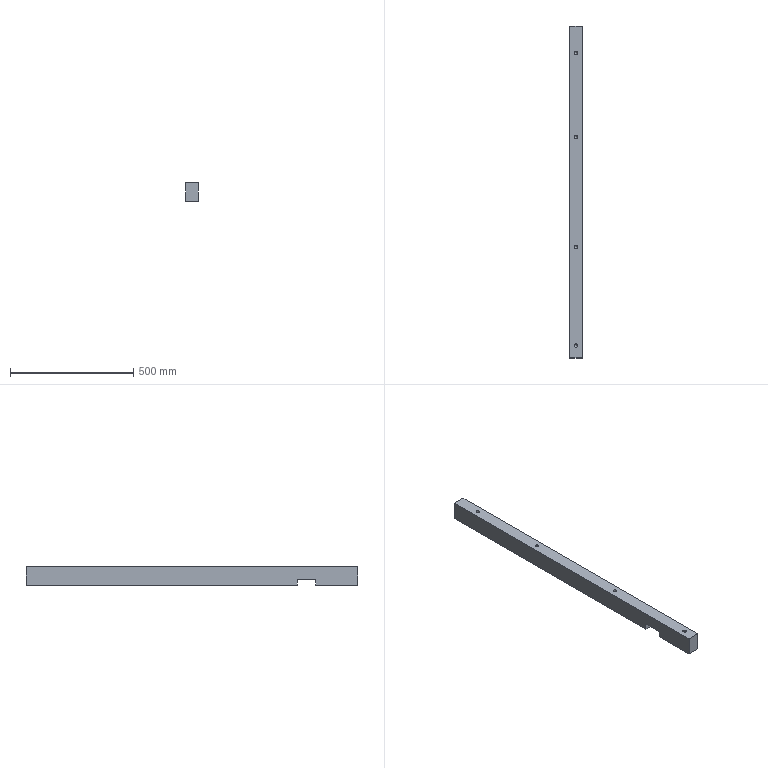Part | NX | features 3 2 | 1 solid | 26 faces | box 50 x 1345 x 75.5 mm | volume 4973309 mm3 | plane 10 | cylinder 8 | cone 8 | commonest cylinder face diameters 14.1 x8
STEP:
#1=CARTESIAN_POINT('',(3150.05,222.5,256.5));
#2=VERTEX_POINT('',#1);
#3=CARTESIAN_POINT('',(3143.,222.5,256.5));
#4=DIRECTION('',(0.,0.,-1.));
#5=DIRECTION('',(1.,0.,0.));
#6=AXIS2_PLACEMENT_3D('',#3,#4,#5);
#7=CIRCLE('',#6,7.05);
#8=EDGE_CURVE('',#2,#2,#7,.T.);
#9=ORIENTED_EDGE('',*,*,#8,.T.);
#10=EDGE_LOOP('',(#9));
#11=FACE_BOUND('',#10,.T.);
#12=CARTESIAN_POINT('',(3150.05,-222.5,256.5));
#13=VERTEX_POINT('',#12);
#14=CARTESIAN_POINT('',(3143.,-222.5,256.5));
#15=DIRECTION('',(0.,0.,-1.));
#16=DIRECTION('',(1.,0.,0.));
#17=AXIS2_PLACEMENT_3D('',#14,#15,#16);
#18=CIRCLE('',#17,7.05);
#19=EDGE_CURVE('',#13,#13,#18,.T.);
#20=ORIENTED_EDGE('',*,*,#19,.T.);
#21=EDGE_LOOP('',(#20));
#22=FACE_BOUND('',#21,.T.);
#23=CARTESIAN_POINT('',(3168.,-672.5,256.5));
#24=VERTEX_POINT('',#23);
#25=CARTESIAN_POINT('',(3168.,672.5,256.5));
#26=VERTEX_POINT('',#25);
#27=CARTESIAN_POINT('',(3168.,193.,256.5));
#28=DIRECTION('',(0.,1.,0.));
#29=VECTOR('',#28,1000.);
#30=LINE('',#27,#29);
#31=EDGE_CURVE('',#24,#26,#30,.T.);
#32=ORIENTED_EDGE('',*,*,#31,.T.);
#33=CARTESIAN_POINT('',(3118.,672.5,256.5));
#34=VERTEX_POINT('',#33);
#35=CARTESIAN_POINT('',(1128.,672.5,256.5));
#36=DIRECTION('',(-1.,0.,0.));
#37=VECTOR('',#36,1000.);
#38=LINE('',#35,#37);
#39=EDGE_CURVE('',#26,#34,#38,.T.);
#40=ORIENTED_EDGE('',*,*,#39,.T.);
#41=CARTESIAN_POINT('',(3118.,-672.5,256.5));
#42=VERTEX_POINT('',#41);
#43=CARTESIAN_POINT('',(3118.,193.,256.5));
#44=DIRECTION('',(0.,-1.,0.));
#45=VECTOR('',#44,1000.);
#46=LINE('',#43,#45);
#47=EDGE_CURVE('',#34,#42,#46,.T.);
#48=ORIENTED_EDGE('',*,*,#47,.T.);
#49=CARTESIAN_POINT('',(1128.,-672.5,256.5));
#50=DIRECTION('',(1.,0.,0.));
#51=VECTOR('',#50,1000.);
#52=LINE('',#49,#51);
#53=EDGE_CURVE('',#42,#24,#52,.T.);
#54=ORIENTED_EDGE('',*,*,#53,.T.);
#55=EDGE_LOOP('',(#32,#40,#48,#54));
#56=FACE_BOUND('',#55,.T.);
#57=CARTESIAN_POINT('',(3150.05,-622.5,256.5));
#58=VERTEX_POINT('',#57);
#59=CARTESIAN_POINT('',(3143.,-622.5,256.5));
#60=DIRECTION('',(0.,0.,-1.));
#61=DIRECTION('',(1.,0.,0.));
#62=AXIS2_PLACEMENT_3D('',#59,#60,#61);
#63=CIRCLE('',#62,7.05);
#64=EDGE_CURVE('',#58,#58,#63,.T.);
#65=ORIENTED_EDGE('',*,*,#64,.T.);
#66=EDGE_LOOP('',(#65));
#67=FACE_BOUND('',#66,.T.);
#68=CARTESIAN_POINT('',(3150.05,562.5,256.5));
#69=VERTEX_POINT('',#68);
#70=CARTESIAN_POINT('',(3143.,562.5,256.5));
#71=DIRECTION('',(0.,0.,-1.));
#72=DIRECTION('',(1.,0.,0.));
#73=AXIS2_PLACEMENT_3D('',#70,#71,#72);
#74=CIRCLE('',#73,7.05);
#75=EDGE_CURVE('',#69,#69,#74,.T.);
#76=ORIENTED_EDGE('',*,*,#75,.T.);
#77=EDGE_LOOP('',(#76));
#78=FACE_BOUND('',#77,.T.);
#79=CARTESIAN_POINT('',(1128.,0.,256.5));
#80=DIRECTION('',(0.,0.,1.));
#81=DIRECTION('',(1.,0.,0.));
#82=AXIS2_PLACEMENT_3D('',#79,#80,#81);
#83=PLANE('',#82);
#84=ADVANCED_FACE('',(#11,#22,#56,#67,#78),#83,.T.);
#85=CARTESIAN_POINT('',(3150.05,-222.5,181.));
#86=VERTEX_POINT('',#85);
#87=CARTESIAN_POINT('',(3143.,-222.5,181.));
#88=DIRECTION('',(0.,0.,1.));
#89=DIRECTION('',(1.,0.,0.));
#90=AXIS2_PLACEMENT_3D('',#87,#88,#89);
#91=CIRCLE('',#90,7.05);
#92=EDGE_CURVE('',#86,#86,#91,.T.);
#93=ORIENTED_EDGE('',*,*,#92,.T.);
#94=EDGE_LOOP('',(#93));
#95=FACE_BOUND('',#94,.T.);
#96=CARTESIAN_POINT('',(3118.,-426.,181.));
#97=VERTEX_POINT('',#96);
#98=CARTESIAN_POINT('',(3168.,-426.,181.));
#99=VERTEX_POINT('',#98);
#100=CARTESIAN_POINT('',(1898.,-426.,181.));
#101=DIRECTION('',(1.,0.,0.));
#102=VECTOR('',#101,1000.);
#103=LINE('',#100,#102);
#104=EDGE_CURVE('',#97,#99,#103,.T.);
#105=ORIENTED_EDGE('',*,*,#104,.F.);
#106=CARTESIAN_POINT('',(3118.,672.5,181.));
#107=VERTEX_POINT('',#106);
#108=CARTESIAN_POINT('',(3118.,193.,181.));
#109=DIRECTION('',(0.,1.,0.));
#110=VECTOR('',#109,1000.);
#111=LINE('',#108,#110);
#112=EDGE_CURVE('',#97,#107,#111,.T.);
#113=ORIENTED_EDGE('',*,*,#112,.T.);
#114=CARTESIAN_POINT('',(3168.,672.5,181.));
#115=VERTEX_POINT('',#114);
#116=CARTESIAN_POINT('',(3168.,672.5,181.));
#117=DIRECTION('',(-1.,0.,0.));
#118=VECTOR('',#117,1000.);
#119=LINE('',#116,#118);
#120=EDGE_CURVE('',#115,#107,#119,.T.);
#121=ORIENTED_EDGE('',*,*,#120,.F.);
#122=CARTESIAN_POINT('',(3168.,193.,181.));
#123=DIRECTION('',(0.,-1.,0.));
#124=VECTOR('',#123,1000.);
#125=LINE('',#122,#124);
#126=EDGE_CURVE('',#115,#99,#125,.T.);
#127=ORIENTED_EDGE('',*,*,#126,.T.);
#128=EDGE_LOOP('',(#105,#113,#121,#127));
#129=FACE_BOUND('',#128,.T.);
#130=CARTESIAN_POINT('',(3150.05,222.5,181.));
#131=VERTEX_POINT('',#130);
#132=CARTESIAN_POINT('',(3143.,222.5,181.));
#133=DIRECTION('',(0.,0.,1.));
#134=DIRECTION('',(1.,0.,0.));
#135=AXIS2_PLACEMENT_3D('',#132,#133,#134);
#136=CIRCLE('',#135,7.05);
#137=EDGE_CURVE('',#131,#131,#136,.T.);
#138=ORIENTED_EDGE('',*,*,#137,.T.);
#139=EDGE_LOOP('',(#138));
#140=FACE_BOUND('',#139,.T.);
#141=CARTESIAN_POINT('',(3150.05,562.5,181.));
#142=VERTEX_POINT('',#141);
#143=CARTESIAN_POINT('',(3143.,562.5,181.));
#144=DIRECTION('',(0.,0.,1.));
#145=DIRECTION('',(1.,0.,0.));
#146=AXIS2_PLACEMENT_3D('',#143,#144,#145);
#147=CIRCLE('',#146,7.05);
#148=EDGE_CURVE('',#142,#142,#147,.T.);
#149=ORIENTED_EDGE('',*,*,#148,.T.);
#150=EDGE_LOOP('',(#149));
#151=FACE_BOUND('',#150,.T.);
#152=CARTESIAN_POINT('',(1898.,193.,181.));
#153=DIRECTION('',(0.,0.,-1.));
#154=DIRECTION('',(1.,0.,0.));
#155=AXIS2_PLACEMENT_3D('',#152,#153,#154);
#156=PLANE('',#155);
#157=ADVANCED_FACE('',(#95,#129,#140,#151),#156,.T.);
#158=CARTESIAN_POINT('',(3168.,-502.,181.));
#159=VERTEX_POINT('',#158);
#160=CARTESIAN_POINT('',(3118.,-502.,181.));
#161=VERTEX_POINT('',#160);
#162=CARTESIAN_POINT('',(1898.,-502.,181.));
#163=DIRECTION('',(-1.,0.,0.));
#164=VECTOR('',#163,1000.);
#165=LINE('',#162,#164);
#166=EDGE_CURVE('',#159,#161,#165,.T.);
#167=ORIENTED_EDGE('',*,*,#166,.F.);
#168=CARTESIAN_POINT('',(3168.,-672.5,181.));
#169=VERTEX_POINT('',#168);
#170=CARTESIAN_POINT('',(3168.,193.,181.));
#171=DIRECTION('',(0.,-1.,0.));
#172=VECTOR('',#171,1000.);
#173=LINE('',#170,#172);
#174=EDGE_CURVE('',#159,#169,#173,.T.);
#175=ORIENTED_EDGE('',*,*,#174,.T.);
#176=CARTESIAN_POINT('',(3118.,-672.5,181.));
#177=VERTEX_POINT('',#176);
#178=CARTESIAN_POINT('',(265.5,-672.5,181.));
#179=DIRECTION('',(1.,0.,0.));
#180=VECTOR('',#179,1000.);
#181=LINE('',#178,#180);
#182=EDGE_CURVE('',#177,#169,#181,.T.);
#183=ORIENTED_EDGE('',*,*,#182,.F.);
#184=CARTESIAN_POINT('',(3118.,193.,181.));
#185=DIRECTION('',(0.,1.,0.));
#186=VECTOR('',#185,1000.);
#187=LINE('',#184,#186);
#188=EDGE_CURVE('',#177,#161,#187,.T.);
#189=ORIENTED_EDGE('',*,*,#188,.T.);
#190=EDGE_LOOP('',(#167,#175,#183,#189));
#191=FACE_BOUND('',#190,.T.);
#192=CARTESIAN_POINT('',(3150.05,-622.5,181.));
#193=VERTEX_POINT('',#192);
#194=CARTESIAN_POINT('',(3143.,-622.5,181.));
#195=DIRECTION('',(0.,0.,1.));
#196=DIRECTION('',(1.,0.,0.));
#197=AXIS2_PLACEMENT_3D('',#194,#195,#196);
#198=CIRCLE('',#197,7.05);
#199=EDGE_CURVE('',#193,#193,#198,.T.);
#200=ORIENTED_EDGE('',*,*,#199,.T.);
#201=EDGE_LOOP('',(#200));
#202=FACE_BOUND('',#201,.T.);
#203=CARTESIAN_POINT('',(1898.,193.,181.));
#204=DIRECTION('',(0.,0.,-1.));
#205=DIRECTION('',(1.,0.,0.));
#206=AXIS2_PLACEMENT_3D('',#203,#204,#205);
#207=PLANE('',#206);
#208=ADVANCED_FACE('',(#191,#202),#207,.T.);
#209=CARTESIAN_POINT('',(3168.,-502.,205.));
#210=VERTEX_POINT('',#209);
#211=CARTESIAN_POINT('',(3168.,-502.,-1.5));
#212=DIRECTION('',(0.,0.,-1.));
#213=VECTOR('',#212,1000.);
#214=LINE('',#211,#213);
#215=EDGE_CURVE('',#210,#159,#214,.T.);
#216=ORIENTED_EDGE('',*,*,#215,.F.);
#217=CARTESIAN_POINT('',(3168.,-426.,205.));
#218=VERTEX_POINT('',#217);
#219=CARTESIAN_POINT('',(3168.,193.,205.));
#220=DIRECTION('',(0.,-1.,0.));
#221=VECTOR('',#220,1000.);
#222=LINE('',#219,#221);
#223=EDGE_CURVE('',#218,#210,#222,.T.);
#224=ORIENTED_EDGE('',*,*,#223,.F.);
#225=CARTESIAN_POINT('',(3168.,-426.,-1.5));
#226=DIRECTION('',(0.,0.,1.));
#227=VECTOR('',#226,1000.);
#228=LINE('',#225,#227);
#229=EDGE_CURVE('',#99,#218,#228,.T.);
#230=ORIENTED_EDGE('',*,*,#229,.F.);
#231=ORIENTED_EDGE('',*,*,#126,.F.);
#232=CARTESIAN_POINT('',(3168.,672.5,231.5));
#233=DIRECTION('',(0.,0.,-1.));
#234=VECTOR('',#233,1000.);
#235=LINE('',#232,#234);
#236=EDGE_CURVE('',#26,#115,#235,.T.);
#237=ORIENTED_EDGE('',*,*,#236,.F.);
#238=ORIENTED_EDGE('',*,*,#31,.F.);
#239=CARTESIAN_POINT('',(3168.,-672.5,-103.));
#240=DIRECTION('',(0.,0.,1.));
#241=VECTOR('',#240,1000.);
#242=LINE('',#239,#241);
#243=EDGE_CURVE('',#169,#24,#242,.T.);
#244=ORIENTED_EDGE('',*,*,#243,.F.);
#245=ORIENTED_EDGE('',*,*,#174,.F.);
#246=EDGE_LOOP('',(#216,#224,#230,#231,#237,#238,#244,#245));
#247=FACE_BOUND('',#246,.T.);
#248=CARTESIAN_POINT('',(3168.,193.,-1.5));
#249=DIRECTION('',(1.,0.,0.));
#250=DIRECTION('',(0.,0.,-1.));
#251=AXIS2_PLACEMENT_3D('',#248,#249,#250);
#252=PLANE('',#251);
#253=ADVANCED_FACE('',(#247),#252,.T.);
#254=CARTESIAN_POINT('',(3118.,-502.,205.));
#255=VERTEX_POINT('',#254);
#256=CARTESIAN_POINT('',(3118.,-502.,-1.5));
#257=DIRECTION('',(0.,0.,1.));
#258=VECTOR('',#257,1000.);
#259=LINE('',#256,#258);
#260=EDGE_CURVE('',#161,#255,#259,.T.);
#261=ORIENTED_EDGE('',*,*,#260,.F.);
#262=ORIENTED_EDGE('',*,*,#188,.F.);
#263=CARTESIAN_POINT('',(3118.,-672.5,-103.));
#264=DIRECTION('',(0.,0.,-1.));
#265=VECTOR('',#264,1000.);
#266=LINE('',#263,#265);
#267=EDGE_CURVE('',#42,#177,#266,.T.);
#268=ORIENTED_EDGE('',*,*,#267,.F.);
#269=ORIENTED_EDGE('',*,*,#47,.F.);
#270=CARTESIAN_POINT('',(3118.,672.5,231.5));
#271=DIRECTION('',(0.,0.,1.));
#272=VECTOR('',#271,1000.);
#273=LINE('',#270,#272);
#274=EDGE_CURVE('',#107,#34,#273,.T.);
#275=ORIENTED_EDGE('',*,*,#274,.F.);
#276=ORIENTED_EDGE('',*,*,#112,.F.);
#277=CARTESIAN_POINT('',(3118.,-426.,205.));
#278=VERTEX_POINT('',#277);
#279=CARTESIAN_POINT('',(3118.,-426.,-1.5));
#280=DIRECTION('',(0.,0.,-1.));
#281=VECTOR('',#280,1000.);
#282=LINE('',#279,#281);
#283=EDGE_CURVE('',#278,#97,#282,.T.);
#284=ORIENTED_EDGE('',*,*,#283,.F.);
#285=CARTESIAN_POINT('',(3118.,193.,205.));
#286=DIRECTION('',(0.,1.,0.));
#287=VECTOR('',#286,1000.);
#288=LINE('',#285,#287);
#289=EDGE_CURVE('',#255,#278,#288,.T.);
#290=ORIENTED_EDGE('',*,*,#289,.F.);
#291=EDGE_LOOP('',(#261,#262,#268,#269,#275,#276,#284,#290));
#292=FACE_BOUND('',#291,.T.);
#293=CARTESIAN_POINT('',(3118.,193.,-1.5));
#294=DIRECTION('',(-1.,0.,0.));
#295=DIRECTION('',(0.,0.,1.));
#296=AXIS2_PLACEMENT_3D('',#293,#294,#295);
#297=PLANE('',#296);
#298=ADVANCED_FACE('',(#292),#297,.T.);
#299=ORIENTED_EDGE('',*,*,#267,.T.);
#300=ORIENTED_EDGE('',*,*,#182,.T.);
#301=ORIENTED_EDGE('',*,*,#243,.T.);
#302=ORIENTED_EDGE('',*,*,#53,.F.);
#303=EDGE_LOOP('',(#299,#300,#301,#302));
#304=FACE_BOUND('',#303,.T.);
#305=CARTESIAN_POINT('',(265.5,-672.5,-103.));
#306=DIRECTION('',(0.,1.,0.));
#307=DIRECTION('',(1.,0.,0.));
#308=AXIS2_PLACEMENT_3D('',#305,#306,#307);
#309=PLANE('',#308);
#310=ADVANCED_FACE('',(#304),#309,.F.);
#311=ORIENTED_EDGE('',*,*,#236,.T.);
#312=ORIENTED_EDGE('',*,*,#120,.T.);
#313=ORIENTED_EDGE('',*,*,#274,.T.);
#314=ORIENTED_EDGE('',*,*,#39,.F.);
#315=EDGE_LOOP('',(#311,#312,#313,#314));
#316=FACE_BOUND('',#315,.T.);
#317=CARTESIAN_POINT('',(3168.,672.5,231.5));
#318=DIRECTION('',(0.,1.,0.));
#319=DIRECTION('',(0.,0.,-1.));
#320=AXIS2_PLACEMENT_3D('',#317,#318,#319);
#321=PLANE('',#320);
#322=ADVANCED_FACE('',(#316),#321,.T.);
#323=ORIENTED_EDGE('',*,*,#223,.T.);
#324=CARTESIAN_POINT('',(3141.,-502.,205.));
#325=DIRECTION('',(1.,0.,0.));
#326=VECTOR('',#325,1000.);
#327=LINE('',#324,#326);
#328=EDGE_CURVE('',#255,#210,#327,.T.);
#329=ORIENTED_EDGE('',*,*,#328,.F.);
#330=ORIENTED_EDGE('',*,*,#289,.T.);
#331=CARTESIAN_POINT('',(3141.,-426.,205.));
#332=DIRECTION('',(-1.,0.,0.));
#333=VECTOR('',#332,1000.);
#334=LINE('',#331,#333);
#335=EDGE_CURVE('',#218,#278,#334,.T.);
#336=ORIENTED_EDGE('',*,*,#335,.F.);
#337=EDGE_LOOP('',(#323,#329,#330,#336));
#338=FACE_BOUND('',#337,.T.);
#339=CARTESIAN_POINT('',(3141.,-464.,205.));
#340=DIRECTION('',(0.,0.,1.));
#341=DIRECTION('',(-1.,0.,0.));
#342=AXIS2_PLACEMENT_3D('',#339,#340,#341);
#343=PLANE('',#342);
#344=ADVANCED_FACE('',(#338),#343,.F.);
#345=ORIENTED_EDGE('',*,*,#215,.T.);
#346=ORIENTED_EDGE('',*,*,#166,.T.);
#347=ORIENTED_EDGE('',*,*,#260,.T.);
#348=ORIENTED_EDGE('',*,*,#328,.T.);
#349=EDGE_LOOP('',(#345,#346,#347,#348));
#350=FACE_BOUND('',#349,.T.);
#351=CARTESIAN_POINT('',(3141.,-502.,25.));
#352=DIRECTION('',(0.,-1.,0.));
#353=DIRECTION('',(0.,0.,1.));
#354=AXIS2_PLACEMENT_3D('',#351,#352,#353);
#355=PLANE('',#354);
#356=ADVANCED_FACE('',(#350),#355,.F.);
#357=ORIENTED_EDGE('',*,*,#229,.T.);
#358=ORIENTED_EDGE('',*,*,#335,.T.);
#359=ORIENTED_EDGE('',*,*,#283,.T.);
#360=ORIENTED_EDGE('',*,*,#104,.T.);
#361=EDGE_LOOP('',(#357,#358,#359,#360));
#362=FACE_BOUND('',#361,.T.);
#363=CARTESIAN_POINT('',(3141.,-426.,25.));
#364=DIRECTION('',(0.,1.,0.));
#365=DIRECTION('',(0.,0.,-1.));
#366=AXIS2_PLACEMENT_3D('',#363,#364,#365);
#367=PLANE('',#366);
#368=ADVANCED_FACE('',(#362),#367,.F.);
#369=CARTESIAN_POINT('',(3150.05,222.5,188.95));
#370=VERTEX_POINT('',#369);
#371=CARTESIAN_POINT('',(3143.,222.5,188.95));
#372=DIRECTION('',(0.,0.,1.));
#373=DIRECTION('',(1.,0.,0.));
#374=AXIS2_PLACEMENT_3D('',#371,#372,#373);
#375=CIRCLE('',#374,7.05);
#376=EDGE_CURVE('',#370,#370,#375,.T.);
#377=ORIENTED_EDGE('',*,*,#376,.T.);
#378=EDGE_LOOP('',(#377));
#379=FACE_BOUND('',#378,.T.);
#380=ORIENTED_EDGE('',*,*,#137,.F.);
#381=EDGE_LOOP('',(#380));
#382=FACE_BOUND('',#381,.T.);
#383=CARTESIAN_POINT('',(3143.,222.5,181.));
#384=DIRECTION('',(0.,0.,1.));
#385=DIRECTION('',(-1.,0.,0.));
#386=AXIS2_PLACEMENT_3D('',#383,#384,#385);
#387=CYLINDRICAL_SURFACE('',#386,7.05);
#388=ADVANCED_FACE('',(#379,#382),#387,.F.);
#389=CARTESIAN_POINT('',(3143.,222.5,196.));
#390=VERTEX_POINT('',#389);
#391=VERTEX_LOOP('',#390);
#392=FACE_BOUND('',#391,.T.);
#393=ORIENTED_EDGE('',*,*,#376,.F.);
#394=EDGE_LOOP('',(#393));
#395=FACE_BOUND('',#394,.T.);
#396=CARTESIAN_POINT('',(3143.,222.5,188.95));
#397=DIRECTION('',(0.,0.,-1.));
#398=DIRECTION('',(1.,0.,0.));
#399=AXIS2_PLACEMENT_3D('',#396,#397,#398);
#400=CONICAL_SURFACE('',#399,7.05,0.7854);
#401=ADVANCED_FACE('',(#392,#395),#400,.F.);
#402=CARTESIAN_POINT('',(3150.05,-622.5,188.95));
#403=VERTEX_POINT('',#402);
#404=CARTESIAN_POINT('',(3143.,-622.5,188.95));
#405=DIRECTION('',(0.,0.,1.));
#406=DIRECTION('',(1.,0.,0.));
#407=AXIS2_PLACEMENT_3D('',#404,#405,#406);
#408=CIRCLE('',#407,7.05);
#409=EDGE_CURVE('',#403,#403,#408,.T.);
#410=ORIENTED_EDGE('',*,*,#409,.T.);
#411=EDGE_LOOP('',(#410));
#412=FACE_BOUND('',#411,.T.);
#413=ORIENTED_EDGE('',*,*,#199,.F.);
#414=EDGE_LOOP('',(#413));
#415=FACE_BOUND('',#414,.T.);
#416=CARTESIAN_POINT('',(3143.,-622.5,181.));
#417=DIRECTION('',(0.,0.,1.));
#418=DIRECTION('',(-1.,0.,0.));
#419=AXIS2_PLACEMENT_3D('',#416,#417,#418);
#420=CYLINDRICAL_SURFACE('',#419,7.05);
#421=ADVANCED_FACE('',(#412,#415),#420,.F.);
#422=CARTESIAN_POINT('',(3143.,-622.5,196.));
#423=VERTEX_POINT('',#422);
#424=VERTEX_LOOP('',#423);
#425=FACE_BOUND('',#424,.T.);
#426=ORIENTED_EDGE('',*,*,#409,.F.);
#427=EDGE_LOOP('',(#426));
#428=FACE_BOUND('',#427,.T.);
#429=CARTESIAN_POINT('',(3143.,-622.5,188.95));
#430=DIRECTION('',(0.,0.,-1.));
#431=DIRECTION('',(1.,0.,0.));
#432=AXIS2_PLACEMENT_3D('',#429,#430,#431);
#433=CONICAL_SURFACE('',#432,7.05,0.7854);
#434=ADVANCED_FACE('',(#425,#428),#433,.F.);
#435=CARTESIAN_POINT('',(3150.05,-222.5,188.95));
#436=VERTEX_POINT('',#435);
#437=CARTESIAN_POINT('',(3143.,-222.5,188.95));
#438=DIRECTION('',(0.,0.,1.));
#439=DIRECTION('',(1.,0.,0.));
#440=AXIS2_PLACEMENT_3D('',#437,#438,#439);
#441=CIRCLE('',#440,7.05);
#442=EDGE_CURVE('',#436,#436,#441,.T.);
#443=ORIENTED_EDGE('',*,*,#442,.T.);
#444=EDGE_LOOP('',(#443));
#445=FACE_BOUND('',#444,.T.);
#446=ORIENTED_EDGE('',*,*,#92,.F.);
#447=EDGE_LOOP('',(#446));
#448=FACE_BOUND('',#447,.T.);
#449=CARTESIAN_POINT('',(3143.,-222.5,181.));
#450=DIRECTION('',(0.,0.,1.));
#451=DIRECTION('',(-1.,0.,0.));
#452=AXIS2_PLACEMENT_3D('',#449,#450,#451);
#453=CYLINDRICAL_SURFACE('',#452,7.05);
#454=ADVANCED_FACE('',(#445,#448),#453,.F.);
#455=CARTESIAN_POINT('',(3143.,-222.5,196.));
#456=VERTEX_POINT('',#455);
#457=VERTEX_LOOP('',#456);
#458=FACE_BOUND('',#457,.T.);
#459=ORIENTED_EDGE('',*,*,#442,.F.);
#460=EDGE_LOOP('',(#459));
#461=FACE_BOUND('',#460,.T.);
#462=CARTESIAN_POINT('',(3143.,-222.5,188.95));
#463=DIRECTION('',(0.,0.,-1.));
#464=DIRECTION('',(1.,0.,0.));
#465=AXIS2_PLACEMENT_3D('',#462,#463,#464);
#466=CONICAL_SURFACE('',#465,7.05,0.7854);
#467=ADVANCED_FACE('',(#458,#461),#466,.F.);
#468=CARTESIAN_POINT('',(3150.05,562.5,188.95));
#469=VERTEX_POINT('',#468);
#470=CARTESIAN_POINT('',(3143.,562.5,188.95));
#471=DIRECTION('',(0.,0.,1.));
#472=DIRECTION('',(1.,0.,0.));
#473=AXIS2_PLACEMENT_3D('',#470,#471,#472);
#474=CIRCLE('',#473,7.05);
#475=EDGE_CURVE('',#469,#469,#474,.T.);
#476=ORIENTED_EDGE('',*,*,#475,.T.);
#477=EDGE_LOOP('',(#476));
#478=FACE_BOUND('',#477,.T.);
#479=ORIENTED_EDGE('',*,*,#148,.F.);
#480=EDGE_LOOP('',(#479));
#481=FACE_BOUND('',#480,.T.);
#482=CARTESIAN_POINT('',(3143.,562.5,181.));
#483=DIRECTION('',(0.,0.,1.));
#484=DIRECTION('',(-1.,0.,0.));
#485=AXIS2_PLACEMENT_3D('',#482,#483,#484);
#486=CYLINDRICAL_SURFACE('',#485,7.05);
#487=ADVANCED_FACE('',(#478,#481),#486,.F.);
#488=CARTESIAN_POINT('',(3143.,562.5,196.));
#489=VERTEX_POINT('',#488);
#490=VERTEX_LOOP('',#489);
#491=FACE_BOUND('',#490,.T.);
#492=ORIENTED_EDGE('',*,*,#475,.F.);
#493=EDGE_LOOP('',(#492));
#494=FACE_BOUND('',#493,.T.);
#495=CARTESIAN_POINT('',(3143.,562.5,188.95));
#496=DIRECTION('',(0.,0.,-1.));
#497=DIRECTION('',(1.,0.,0.));
#498=AXIS2_PLACEMENT_3D('',#495,#496,#497);
#499=CONICAL_SURFACE('',#498,7.05,0.7854);
#500=ADVANCED_FACE('',(#491,#494),#499,.F.);
#501=CARTESIAN_POINT('',(3135.95,-222.5,248.55));
#502=VERTEX_POINT('',#501);
#503=CARTESIAN_POINT('',(3143.,-222.5,248.55));
#504=DIRECTION('',(0.,0.,-1.));
#505=DIRECTION('',(-1.,0.,0.));
#506=AXIS2_PLACEMENT_3D('',#503,#504,#505);
#507=CIRCLE('',#506,7.05);
#508=EDGE_CURVE('',#502,#502,#507,.T.);
#509=ORIENTED_EDGE('',*,*,#508,.T.);
#510=EDGE_LOOP('',(#509));
#511=FACE_BOUND('',#510,.T.);
#512=ORIENTED_EDGE('',*,*,#19,.F.);
#513=EDGE_LOOP('',(#512));
#514=FACE_BOUND('',#513,.T.);
#515=CARTESIAN_POINT('',(3143.,-222.5,256.5));
#516=DIRECTION('',(0.,0.,-1.));
#517=DIRECTION('',(-1.,0.,0.));
#518=AXIS2_PLACEMENT_3D('',#515,#516,#517);
#519=CYLINDRICAL_SURFACE('',#518,7.05);
#520=ADVANCED_FACE('',(#511,#514),#519,.F.);
#521=CARTESIAN_POINT('',(3143.,-222.5,241.5));
#522=VERTEX_POINT('',#521);
#523=VERTEX_LOOP('',#522);
#524=FACE_BOUND('',#523,.T.);
#525=ORIENTED_EDGE('',*,*,#508,.F.);
#526=EDGE_LOOP('',(#525));
#527=FACE_BOUND('',#526,.T.);
#528=CARTESIAN_POINT('',(3143.,-222.5,248.55));
#529=DIRECTION('',(0.,0.,1.));
#530=DIRECTION('',(-1.,0.,0.));
#531=AXIS2_PLACEMENT_3D('',#528,#529,#530);
#532=CONICAL_SURFACE('',#531,7.05,0.7854);
#533=ADVANCED_FACE('',(#524,#527),#532,.F.);
#534=CARTESIAN_POINT('',(3135.95,-622.5,248.55));
#535=VERTEX_POINT('',#534);
#536=CARTESIAN_POINT('',(3143.,-622.5,248.55));
#537=DIRECTION('',(0.,0.,-1.));
#538=DIRECTION('',(-1.,0.,0.));
#539=AXIS2_PLACEMENT_3D('',#536,#537,#538);
#540=CIRCLE('',#539,7.05);
#541=EDGE_CURVE('',#535,#535,#540,.T.);
#542=ORIENTED_EDGE('',*,*,#541,.T.);
#543=EDGE_LOOP('',(#542));
#544=FACE_BOUND('',#543,.T.);
#545=ORIENTED_EDGE('',*,*,#64,.F.);
#546=EDGE_LOOP('',(#545));
#547=FACE_BOUND('',#546,.T.);
#548=CARTESIAN_POINT('',(3143.,-622.5,256.5));
#549=DIRECTION('',(0.,0.,-1.));
#550=DIRECTION('',(-1.,0.,0.));
#551=AXIS2_PLACEMENT_3D('',#548,#549,#550);
#552=CYLINDRICAL_SURFACE('',#551,7.05);
#553=ADVANCED_FACE('',(#544,#547),#552,.F.);
#554=CARTESIAN_POINT('',(3143.,-622.5,241.5));
#555=VERTEX_POINT('',#554);
#556=VERTEX_LOOP('',#555);
#557=FACE_BOUND('',#556,.T.);
#558=ORIENTED_EDGE('',*,*,#541,.F.);
#559=EDGE_LOOP('',(#558));
#560=FACE_BOUND('',#559,.T.);
#561=CARTESIAN_POINT('',(3143.,-622.5,248.55));
#562=DIRECTION('',(0.,0.,1.));
#563=DIRECTION('',(-1.,0.,0.));
#564=AXIS2_PLACEMENT_3D('',#561,#562,#563);
#565=CONICAL_SURFACE('',#564,7.05,0.7854);
#566=ADVANCED_FACE('',(#557,#560),#565,.F.);
#567=CARTESIAN_POINT('',(3135.95,222.5,248.55));
#568=VERTEX_POINT('',#567);
#569=CARTESIAN_POINT('',(3143.,222.5,248.55));
#570=DIRECTION('',(0.,0.,-1.));
#571=DIRECTION('',(-1.,0.,0.));
#572=AXIS2_PLACEMENT_3D('',#569,#570,#571);
#573=CIRCLE('',#572,7.05);
#574=EDGE_CURVE('',#568,#568,#573,.T.);
#575=ORIENTED_EDGE('',*,*,#574,.T.);
#576=EDGE_LOOP('',(#575));
#577=FACE_BOUND('',#576,.T.);
#578=ORIENTED_EDGE('',*,*,#8,.F.);
#579=EDGE_LOOP('',(#578));
#580=FACE_BOUND('',#579,.T.);
#581=CARTESIAN_POINT('',(3143.,222.5,256.5));
#582=DIRECTION('',(0.,0.,-1.));
#583=DIRECTION('',(-1.,0.,0.));
#584=AXIS2_PLACEMENT_3D('',#581,#582,#583);
#585=CYLINDRICAL_SURFACE('',#584,7.05);
#586=ADVANCED_FACE('',(#577,#580),#585,.F.);
#587=CARTESIAN_POINT('',(3143.,222.5,241.5));
#588=VERTEX_POINT('',#587);
#589=VERTEX_LOOP('',#588);
#590=FACE_BOUND('',#589,.T.);
#591=ORIENTED_EDGE('',*,*,#574,.F.);
#592=EDGE_LOOP('',(#591));
#593=FACE_BOUND('',#592,.T.);
#594=CARTESIAN_POINT('',(3143.,222.5,248.55));
#595=DIRECTION('',(0.,0.,1.));
#596=DIRECTION('',(-1.,0.,0.));
#597=AXIS2_PLACEMENT_3D('',#594,#595,#596);
#598=CONICAL_SURFACE('',#597,7.05,0.7854);
#599=ADVANCED_FACE('',(#590,#593),#598,.F.);
#600=CARTESIAN_POINT('',(3135.95,562.5,248.55));
#601=VERTEX_POINT('',#600);
#602=CARTESIAN_POINT('',(3143.,562.5,248.55));
#603=DIRECTION('',(0.,0.,-1.));
#604=DIRECTION('',(-1.,0.,0.));
#605=AXIS2_PLACEMENT_3D('',#602,#603,#604);
#606=CIRCLE('',#605,7.05);
#607=EDGE_CURVE('',#601,#601,#606,.T.);
#608=ORIENTED_EDGE('',*,*,#607,.T.);
#609=EDGE_LOOP('',(#608));
#610=FACE_BOUND('',#609,.T.);
#611=ORIENTED_EDGE('',*,*,#75,.F.);
#612=EDGE_LOOP('',(#611));
#613=FACE_BOUND('',#612,.T.);
#614=CARTESIAN_POINT('',(3143.,562.5,256.5));
#615=DIRECTION('',(0.,0.,-1.));
#616=DIRECTION('',(-1.,0.,0.));
#617=AXIS2_PLACEMENT_3D('',#614,#615,#616);
#618=CYLINDRICAL_SURFACE('',#617,7.05);
#619=ADVANCED_FACE('',(#610,#613),#618,.F.);
#620=CARTESIAN_POINT('',(3143.,562.5,241.5));
#621=VERTEX_POINT('',#620);
#622=VERTEX_LOOP('',#621);
#623=FACE_BOUND('',#622,.T.);
#624=ORIENTED_EDGE('',*,*,#607,.F.);
#625=EDGE_LOOP('',(#624));
#626=FACE_BOUND('',#625,.T.);
#627=CARTESIAN_POINT('',(3143.,562.5,248.55));
#628=DIRECTION('',(0.,0.,1.));
#629=DIRECTION('',(-1.,0.,0.));
#630=AXIS2_PLACEMENT_3D('',#627,#628,#629);
#631=CONICAL_SURFACE('',#630,7.05,0.7854);
#632=ADVANCED_FACE('',(#623,#626),#631,.F.);
#633=CLOSED_SHELL('',(#84,#157,#208,#253,#298,#310,#322,#344,#356,#368,#388,#401,#421,#434,#454,#467,#487,#500,#520,#533,#553,#566,#586,#599,#619,#632));
#634=MANIFOLD_SOLID_BREP('',#633);
#635=(LENGTH_UNIT()NAMED_UNIT(*)SI_UNIT(.MILLI.,.METRE.));
#636=UNCERTAINTY_MEASURE_WITH_UNIT(LENGTH_MEASURE(0.00001),#635,'','');
#637=(NAMED_UNIT(*)PLANE_ANGLE_UNIT()SI_UNIT($,.RADIAN.));
#638=(NAMED_UNIT(*)SI_UNIT($,.STERADIAN.)SOLID_ANGLE_UNIT());
#639=(GEOMETRIC_REPRESENTATION_CONTEXT(3)GLOBAL_UNCERTAINTY_ASSIGNED_CONTEXT((#636))GLOBAL_UNIT_ASSIGNED_CONTEXT((#635,#637,#638))REPRESENTATION_CONTEXT('',''));
#640=ADVANCED_BREP_SHAPE_REPRESENTATION('',(#634),#639);